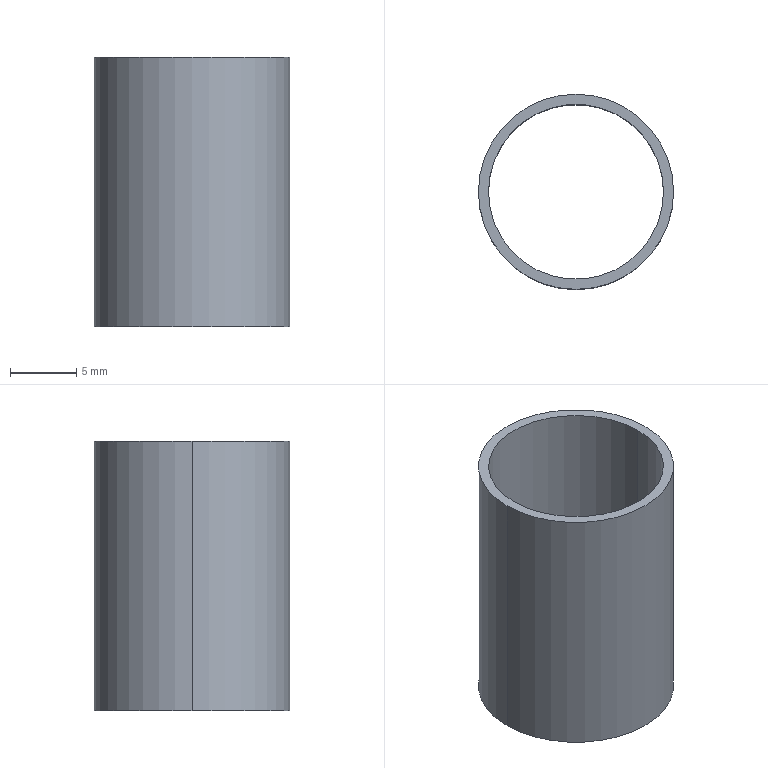Part | SolidWorks | features Extrusion 1, Scale 1 | 1 solid | 6 faces | box 14.732 x 14.732 x 20.32 mm | volume 679.556 mm3 | cylinder 4 | plane 2 | commonest cylinder face diameters 13.208 x2 14.732 x2
STEP:
#1=CARTESIAN_POINT('',(-6.604,0.,20.32));
#2=VERTEX_POINT('',#1);
#3=CARTESIAN_POINT('',(6.604,0.,20.32));
#4=VERTEX_POINT('',#3);
#5=CARTESIAN_POINT('',(0.,0.,20.32));
#6=DIRECTION('',(0.,0.,1.));
#7=DIRECTION('',(1.,0.,0.));
#8=AXIS2_PLACEMENT_3D('',#5,#6,#7);
#9=CIRCLE('',#8,6.604);
#10=EDGE_CURVE('',#2,#4,#9,.T.);
#11=ORIENTED_EDGE('',*,*,#10,.T.);
#12=CARTESIAN_POINT('',(6.604,0.,0.));
#13=VERTEX_POINT('',#12);
#14=CARTESIAN_POINT('',(6.604,0.,20.32));
#15=DIRECTION('',(0.,0.,-1.));
#16=VECTOR('',#15,1000.);
#17=LINE('',#14,#16);
#18=EDGE_CURVE('',#4,#13,#17,.T.);
#19=ORIENTED_EDGE('',*,*,#18,.T.);
#20=CARTESIAN_POINT('',(-6.604,0.,0.));
#21=VERTEX_POINT('',#20);
#22=CARTESIAN_POINT('',(0.,0.,0.));
#23=DIRECTION('',(0.,0.,1.));
#24=DIRECTION('',(1.,0.,0.));
#25=AXIS2_PLACEMENT_3D('',#22,#23,#24);
#26=CIRCLE('',#25,6.604);
#27=EDGE_CURVE('',#21,#13,#26,.T.);
#28=ORIENTED_EDGE('',*,*,#27,.F.);
#29=CARTESIAN_POINT('',(-6.604,0.,20.32));
#30=DIRECTION('',(0.,0.,-1.));
#31=VECTOR('',#30,1000.);
#32=LINE('',#29,#31);
#33=EDGE_CURVE('',#2,#21,#32,.T.);
#34=ORIENTED_EDGE('',*,*,#33,.F.);
#35=EDGE_LOOP('',(#11,#19,#28,#34));
#36=FACE_OUTER_BOUND('',#35,.T.);
#37=CARTESIAN_POINT('',(0.,0.,20.32));
#38=DIRECTION('',(0.,0.,-1.));
#39=DIRECTION('',(-1.,0.,0.));
#40=AXIS2_PLACEMENT_3D('',#37,#38,#39);
#41=CYLINDRICAL_SURFACE('',#40,6.604);
#42=ADVANCED_FACE('',(#36),#41,.F.);
#43=CARTESIAN_POINT('',(7.366,0.,20.32));
#44=VERTEX_POINT('',#43);
#45=CARTESIAN_POINT('',(-7.366,0.,20.32));
#46=VERTEX_POINT('',#45);
#47=CARTESIAN_POINT('',(0.,0.,20.32));
#48=DIRECTION('',(0.,0.,1.));
#49=DIRECTION('',(1.,0.,0.));
#50=AXIS2_PLACEMENT_3D('',#47,#48,#49);
#51=CIRCLE('',#50,7.366);
#52=EDGE_CURVE('',#44,#46,#51,.T.);
#53=ORIENTED_EDGE('',*,*,#52,.F.);
#54=CARTESIAN_POINT('',(7.366,0.,0.));
#55=VERTEX_POINT('',#54);
#56=CARTESIAN_POINT('',(7.366,0.,20.32));
#57=DIRECTION('',(0.,0.,-1.));
#58=VECTOR('',#57,1000.);
#59=LINE('',#56,#58);
#60=EDGE_CURVE('',#44,#55,#59,.T.);
#61=ORIENTED_EDGE('',*,*,#60,.T.);
#62=CARTESIAN_POINT('',(-7.366,0.,0.));
#63=VERTEX_POINT('',#62);
#64=CARTESIAN_POINT('',(0.,0.,0.));
#65=DIRECTION('',(0.,0.,1.));
#66=DIRECTION('',(1.,0.,0.));
#67=AXIS2_PLACEMENT_3D('',#64,#65,#66);
#68=CIRCLE('',#67,7.366);
#69=EDGE_CURVE('',#55,#63,#68,.T.);
#70=ORIENTED_EDGE('',*,*,#69,.T.);
#71=CARTESIAN_POINT('',(-7.366,0.,20.32));
#72=DIRECTION('',(0.,0.,-1.));
#73=VECTOR('',#72,1000.);
#74=LINE('',#71,#73);
#75=EDGE_CURVE('',#46,#63,#74,.T.);
#76=ORIENTED_EDGE('',*,*,#75,.F.);
#77=EDGE_LOOP('',(#53,#61,#70,#76));
#78=FACE_OUTER_BOUND('',#77,.T.);
#79=CARTESIAN_POINT('',(0.,0.,20.32));
#80=DIRECTION('',(0.,0.,-1.));
#81=DIRECTION('',(-1.,0.,0.));
#82=AXIS2_PLACEMENT_3D('',#79,#80,#81);
#83=CYLINDRICAL_SURFACE('',#82,7.366);
#84=ADVANCED_FACE('',(#78),#83,.T.);
#85=CARTESIAN_POINT('',(0.,0.,20.32));
#86=DIRECTION('',(0.,0.,1.));
#87=DIRECTION('',(1.,0.,0.));
#88=AXIS2_PLACEMENT_3D('',#85,#86,#87);
#89=CIRCLE('',#88,7.366);
#90=EDGE_CURVE('',#46,#44,#89,.T.);
#91=ORIENTED_EDGE('',*,*,#90,.T.);
#92=ORIENTED_EDGE('',*,*,#52,.T.);
#93=EDGE_LOOP('',(#91,#92));
#94=FACE_OUTER_BOUND('',#93,.T.);
#95=ORIENTED_EDGE('',*,*,#10,.F.);
#96=CARTESIAN_POINT('',(0.,0.,20.32));
#97=DIRECTION('',(0.,0.,1.));
#98=DIRECTION('',(1.,0.,0.));
#99=AXIS2_PLACEMENT_3D('',#96,#97,#98);
#100=CIRCLE('',#99,6.604);
#101=EDGE_CURVE('',#4,#2,#100,.T.);
#102=ORIENTED_EDGE('',*,*,#101,.F.);
#103=EDGE_LOOP('',(#95,#102));
#104=FACE_BOUND('',#103,.T.);
#105=CARTESIAN_POINT('',(0.,0.,20.32));
#106=DIRECTION('',(0.,0.,1.));
#107=DIRECTION('',(1.,0.,0.));
#108=AXIS2_PLACEMENT_3D('',#105,#106,#107);
#109=PLANE('',#108);
#110=ADVANCED_FACE('',(#94,#104),#109,.T.);
#111=CARTESIAN_POINT('',(0.,0.,0.));
#112=DIRECTION('',(0.,0.,1.));
#113=DIRECTION('',(1.,0.,0.));
#114=AXIS2_PLACEMENT_3D('',#111,#112,#113);
#115=CIRCLE('',#114,7.366);
#116=EDGE_CURVE('',#63,#55,#115,.T.);
#117=ORIENTED_EDGE('',*,*,#116,.F.);
#118=ORIENTED_EDGE('',*,*,#69,.F.);
#119=EDGE_LOOP('',(#117,#118));
#120=FACE_OUTER_BOUND('',#119,.T.);
#121=ORIENTED_EDGE('',*,*,#27,.T.);
#122=CARTESIAN_POINT('',(0.,0.,0.));
#123=DIRECTION('',(0.,0.,1.));
#124=DIRECTION('',(1.,0.,0.));
#125=AXIS2_PLACEMENT_3D('',#122,#123,#124);
#126=CIRCLE('',#125,6.604);
#127=EDGE_CURVE('',#13,#21,#126,.T.);
#128=ORIENTED_EDGE('',*,*,#127,.T.);
#129=EDGE_LOOP('',(#121,#128));
#130=FACE_BOUND('',#129,.T.);
#131=CARTESIAN_POINT('',(0.,0.,0.));
#132=DIRECTION('',(0.,0.,1.));
#133=DIRECTION('',(1.,0.,0.));
#134=AXIS2_PLACEMENT_3D('',#131,#132,#133);
#135=PLANE('',#134);
#136=ADVANCED_FACE('',(#120,#130),#135,.F.);
#137=ORIENTED_EDGE('',*,*,#60,.F.);
#138=ORIENTED_EDGE('',*,*,#90,.F.);
#139=ORIENTED_EDGE('',*,*,#75,.T.);
#140=ORIENTED_EDGE('',*,*,#116,.T.);
#141=EDGE_LOOP('',(#137,#138,#139,#140));
#142=FACE_OUTER_BOUND('',#141,.T.);
#143=CARTESIAN_POINT('',(0.,0.,20.32));
#144=DIRECTION('',(0.,0.,-1.));
#145=DIRECTION('',(-1.,0.,0.));
#146=AXIS2_PLACEMENT_3D('',#143,#144,#145);
#147=CYLINDRICAL_SURFACE('',#146,7.366);
#148=ADVANCED_FACE('',(#142),#147,.T.);
#149=ORIENTED_EDGE('',*,*,#18,.F.);
#150=ORIENTED_EDGE('',*,*,#101,.T.);
#151=ORIENTED_EDGE('',*,*,#33,.T.);
#152=ORIENTED_EDGE('',*,*,#127,.F.);
#153=EDGE_LOOP('',(#149,#150,#151,#152));
#154=FACE_OUTER_BOUND('',#153,.T.);
#155=CARTESIAN_POINT('',(0.,0.,20.32));
#156=DIRECTION('',(0.,0.,-1.));
#157=DIRECTION('',(-1.,0.,0.));
#158=AXIS2_PLACEMENT_3D('',#155,#156,#157);
#159=CYLINDRICAL_SURFACE('',#158,6.604);
#160=ADVANCED_FACE('',(#154),#159,.F.);
#161=CLOSED_SHELL('',(#42,#84,#110,#136,#148,#160));
#162=MANIFOLD_SOLID_BREP('',#161);
#163=CARTESIAN_POINT('',(0.,0.,0.));
#164=DIRECTION('',(0.,0.,1.));
#165=DIRECTION('',(1.,0.,0.));
#166=AXIS2_PLACEMENT_3D('',#163,#164,#165);
#167=(LENGTH_UNIT()NAMED_UNIT(*)SI_UNIT(.MILLI.,.METRE.));
#168=UNCERTAINTY_MEASURE_WITH_UNIT(LENGTH_MEASURE(0.00001),#167,'','');
#169=(NAMED_UNIT(*)PLANE_ANGLE_UNIT()SI_UNIT($,.RADIAN.));
#170=(NAMED_UNIT(*)SI_UNIT($,.STERADIAN.)SOLID_ANGLE_UNIT());
#171=(GEOMETRIC_REPRESENTATION_CONTEXT(3)GLOBAL_UNCERTAINTY_ASSIGNED_CONTEXT((#168))GLOBAL_UNIT_ASSIGNED_CONTEXT((#167,#169,#170))REPRESENTATION_CONTEXT('',''));
#172=ADVANCED_BREP_SHAPE_REPRESENTATION('',(#162,#166),#171);